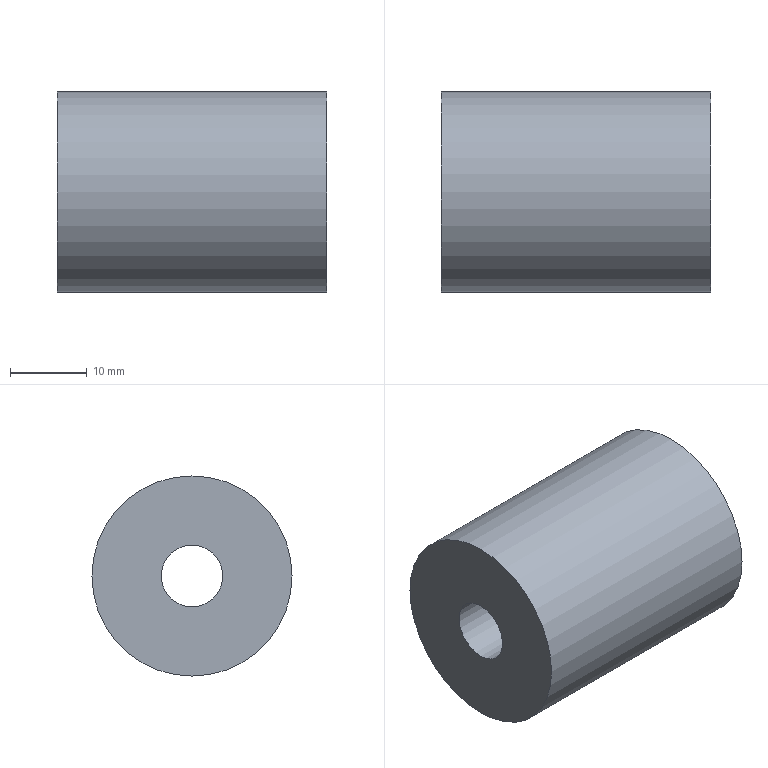Part | NX | 1 solid | 4 faces | box 35 x 26 x 26 mm | volume 16823 mm3 | cylinder 2 | plane 2 | commonest cylinder face diameters 8 x1 26 x1
STEP:
#1=CARTESIAN_POINT('',(17.5,0.,-13.));
#2=VERTEX_POINT('',#1);
#3=CARTESIAN_POINT('',(17.5,0.,0.));
#4=DIRECTION('',(1.,0.,0.));
#5=DIRECTION('',(0.,0.,-1.));
#6=AXIS2_PLACEMENT_3D('',#3,#4,#5);
#7=CIRCLE('',#6,13.);
#8=EDGE_CURVE('',#2,#2,#7,.T.);
#9=ORIENTED_EDGE('',*,*,#8,.F.);
#10=EDGE_LOOP('',(#9));
#11=FACE_BOUND('',#10,.T.);
#12=CARTESIAN_POINT('',(-17.5,0.,-13.));
#13=VERTEX_POINT('',#12);
#14=CARTESIAN_POINT('',(-17.5,0.,0.));
#15=DIRECTION('',(1.,0.,0.));
#16=DIRECTION('',(0.,0.,-1.));
#17=AXIS2_PLACEMENT_3D('',#14,#15,#16);
#18=CIRCLE('',#17,13.);
#19=EDGE_CURVE('',#13,#13,#18,.T.);
#20=ORIENTED_EDGE('',*,*,#19,.T.);
#21=EDGE_LOOP('',(#20));
#22=FACE_BOUND('',#21,.T.);
#23=CARTESIAN_POINT('',(17.5,0.,0.));
#24=DIRECTION('',(-1.,0.,0.));
#25=DIRECTION('',(0.,0.,1.));
#26=AXIS2_PLACEMENT_3D('',#23,#24,#25);
#27=CYLINDRICAL_SURFACE('',#26,13.);
#28=ADVANCED_FACE('',(#11,#22),#27,.T.);
#29=CARTESIAN_POINT('',(17.5,0.,-4.));
#30=VERTEX_POINT('',#29);
#31=CARTESIAN_POINT('',(17.5,0.,0.));
#32=DIRECTION('',(1.,0.,0.));
#33=DIRECTION('',(0.,0.,-1.));
#34=AXIS2_PLACEMENT_3D('',#31,#32,#33);
#35=CIRCLE('',#34,4.);
#36=EDGE_CURVE('',#30,#30,#35,.T.);
#37=ORIENTED_EDGE('',*,*,#36,.F.);
#38=EDGE_LOOP('',(#37));
#39=FACE_BOUND('',#38,.T.);
#40=ORIENTED_EDGE('',*,*,#8,.T.);
#41=EDGE_LOOP('',(#40));
#42=FACE_BOUND('',#41,.T.);
#43=CARTESIAN_POINT('',(17.5,0.,0.));
#44=DIRECTION('',(1.,0.,0.));
#45=DIRECTION('',(0.,0.,-1.));
#46=AXIS2_PLACEMENT_3D('',#43,#44,#45);
#47=PLANE('',#46);
#48=ADVANCED_FACE('',(#39,#42),#47,.T.);
#49=CARTESIAN_POINT('',(-17.5,0.,-4.));
#50=VERTEX_POINT('',#49);
#51=CARTESIAN_POINT('',(-17.5,0.,0.));
#52=DIRECTION('',(1.,0.,0.));
#53=DIRECTION('',(0.,0.,-1.));
#54=AXIS2_PLACEMENT_3D('',#51,#52,#53);
#55=CIRCLE('',#54,4.);
#56=EDGE_CURVE('',#50,#50,#55,.T.);
#57=ORIENTED_EDGE('',*,*,#56,.T.);
#58=EDGE_LOOP('',(#57));
#59=FACE_BOUND('',#58,.T.);
#60=ORIENTED_EDGE('',*,*,#19,.F.);
#61=EDGE_LOOP('',(#60));
#62=FACE_BOUND('',#61,.T.);
#63=CARTESIAN_POINT('',(-17.5,0.,0.));
#64=DIRECTION('',(1.,0.,0.));
#65=DIRECTION('',(0.,0.,-1.));
#66=AXIS2_PLACEMENT_3D('',#63,#64,#65);
#67=PLANE('',#66);
#68=ADVANCED_FACE('',(#59,#62),#67,.F.);
#69=ORIENTED_EDGE('',*,*,#56,.F.);
#70=EDGE_LOOP('',(#69));
#71=FACE_BOUND('',#70,.T.);
#72=ORIENTED_EDGE('',*,*,#36,.T.);
#73=EDGE_LOOP('',(#72));
#74=FACE_BOUND('',#73,.T.);
#75=CARTESIAN_POINT('',(-17.5,0.,0.));
#76=DIRECTION('',(1.,0.,0.));
#77=DIRECTION('',(0.,0.,-1.));
#78=AXIS2_PLACEMENT_3D('',#75,#76,#77);
#79=CYLINDRICAL_SURFACE('',#78,4.);
#80=ADVANCED_FACE('',(#71,#74),#79,.F.);
#81=CLOSED_SHELL('',(#28,#48,#68,#80));
#82=MANIFOLD_SOLID_BREP('',#81);
#83=(LENGTH_UNIT()NAMED_UNIT(*)SI_UNIT(.MILLI.,.METRE.));
#84=UNCERTAINTY_MEASURE_WITH_UNIT(LENGTH_MEASURE(0.00001),#83,'','');
#85=(NAMED_UNIT(*)PLANE_ANGLE_UNIT()SI_UNIT($,.RADIAN.));
#86=(NAMED_UNIT(*)SI_UNIT($,.STERADIAN.)SOLID_ANGLE_UNIT());
#87=(GEOMETRIC_REPRESENTATION_CONTEXT(3)GLOBAL_UNCERTAINTY_ASSIGNED_CONTEXT((#84))GLOBAL_UNIT_ASSIGNED_CONTEXT((#83,#85,#86))REPRESENTATION_CONTEXT('',''));
#88=ADVANCED_BREP_SHAPE_REPRESENTATION('',(#82),#87);